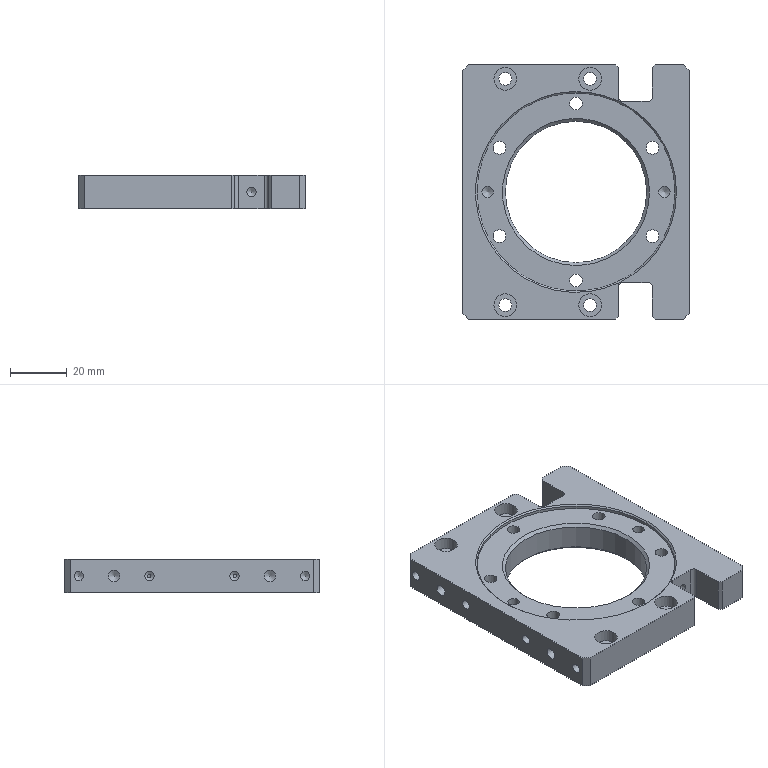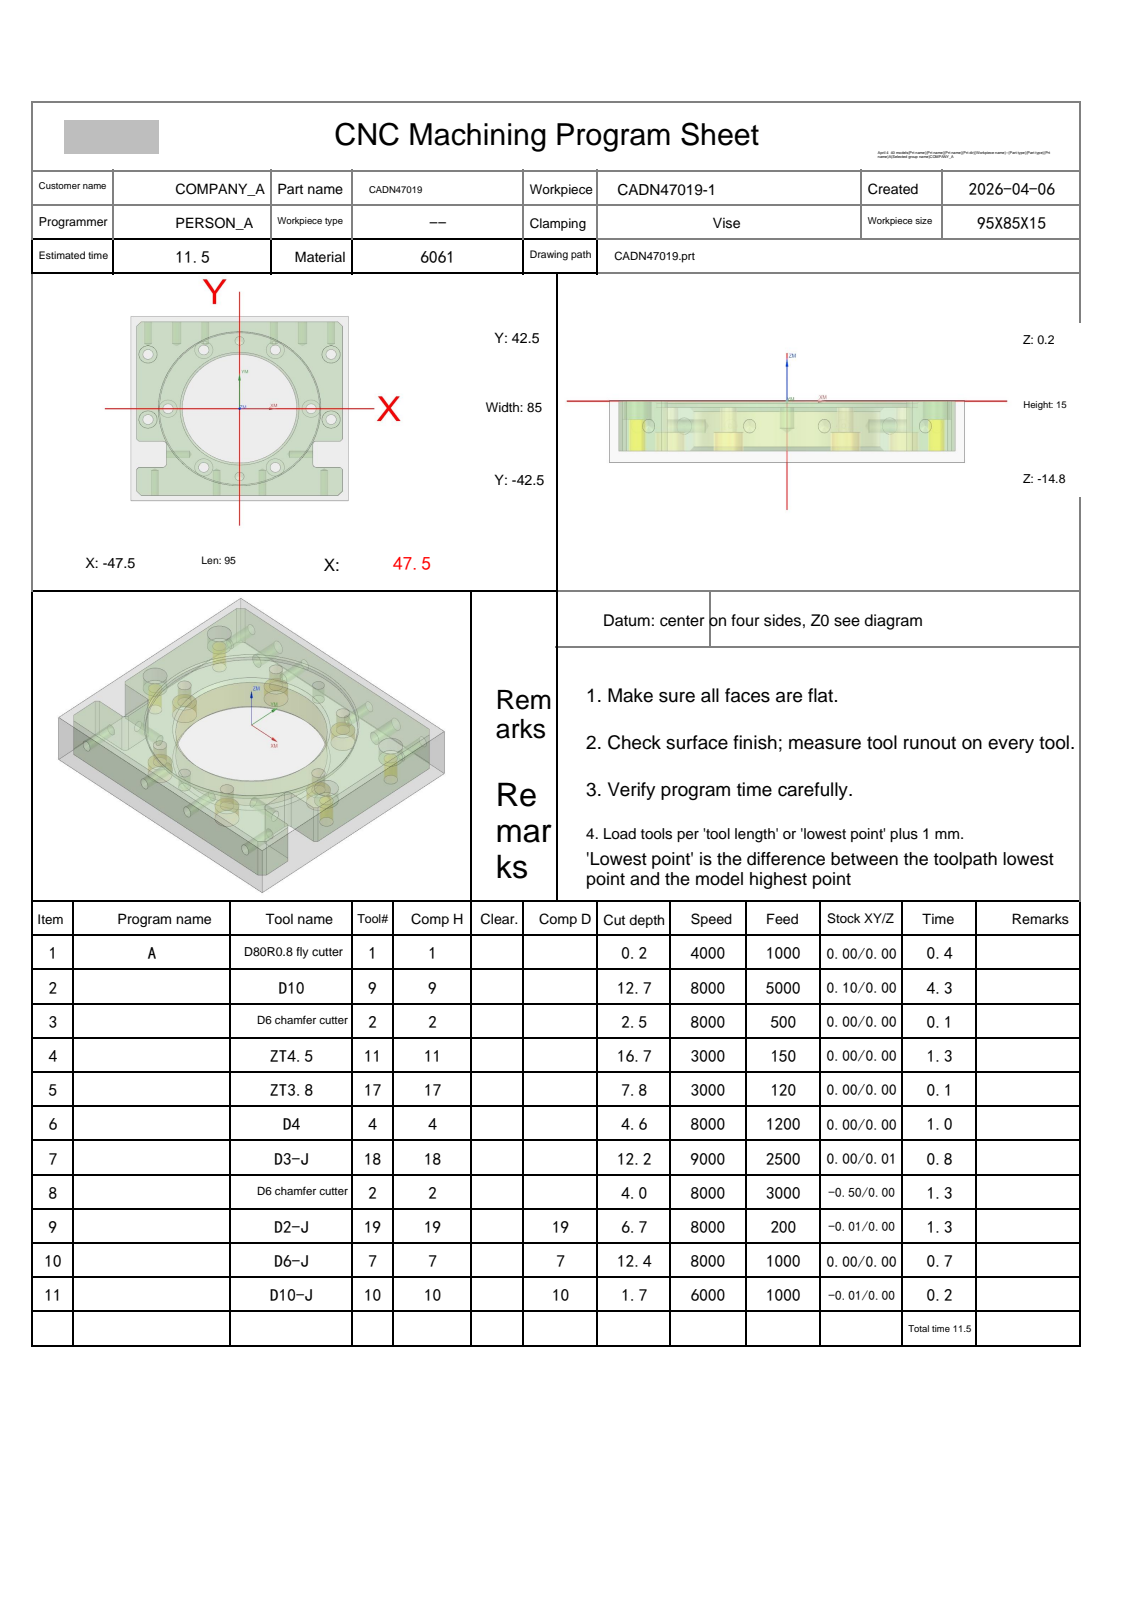NC program | NX | posted by the shop | part box 80 x 90 x 12 mm
Lines 6056 to 6628 of 6628:
N8 T02 M06
(D6 chamfer cutter  D=6. R=0. H=02 ce=0.00 di=0.00)
G00 G90 G54 X-.25 Y42.128 M03 S8000
G43 H02 Z20.
M08
Z2.099
G01 Z-1.5 F3000.
G03 X-.33 Y41.828 I.52 J-.3
X-.03 Y41.308 I.6 J0.0
G01 X0.0 Y41.3
X43.
X43.254 Y41.275
X43.497 Y41.201
X43.722 Y41.081
X43.919 Y40.919
X45.919 Y38.919
X46.081 Y38.722
X46.201 Y38.497
X46.275 Y38.254
X46.3 Y38.
Y-14.
X46.275 Y-14.254
X46.201 Y-14.497
X46.081 Y-14.722
X45.919 Y-14.919
X44.919 Y-15.919
X44.722 Y-16.081
X44.497 Y-16.201
X44.254 Y-16.275
X44. Y-16.3
X33.5
X33.4 Y-16.327
X33.327 Y-16.4
X33.3 Y-16.5
Y-25.5
X33.327 Y-25.6
X33.4 Y-25.673
X33.5 Y-25.7
X44.
X44.254 Y-25.725
X44.497 Y-25.799
X44.722 Y-25.919
X44.919 Y-26.081
X45.919 Y-27.081
X46.081 Y-27.278
X46.201 Y-27.503
X46.275 Y-27.746
X46.3 Y-28.
Y-38.
X46.275 Y-38.254
X46.201 Y-38.497
X46.081 Y-38.722
X45.919 Y-38.919
X43.919 Y-40.919
X43.722 Y-41.081
X43.497 Y-41.201
X43.254 Y-41.275
X43. Y-41.3
X-43.
X-43.254 Y-41.275
X-43.497 Y-41.201
X-43.722 Y-41.081
X-43.919 Y-40.919
X-45.919 Y-38.919
X-46.081 Y-38.722
X-46.201 Y-38.497
X-46.275 Y-38.254
X-46.3 Y-38.
Y-28.
X-46.275 Y-27.746
X-46.201 Y-27.503
X-46.081 Y-27.278
X-45.919 Y-27.081
X-44.919 Y-26.081
X-44.722 Y-25.919
X-44.497 Y-25.799
X-44.254 Y-25.725
X-44. Y-25.7
X-33.5
X-33.4 Y-25.673
X-33.327 Y-25.6
X-33.3 Y-25.5
Y-16.5
X-33.327 Y-16.4
X-33.4 Y-16.327
X-33.5 Y-16.3
X-44.
X-44.254 Y-16.275
X-44.497 Y-16.201
X-44.722 Y-16.081
X-44.919 Y-15.919
X-45.919 Y-14.919
X-46.081 Y-14.722
X-46.201 Y-14.497
X-46.275 Y-14.254
X-46.3 Y-14.
Y38.
X-46.275 Y38.254
X-46.201 Y38.497
X-46.081 Y38.722
X-45.919 Y38.919
X-43.919 Y40.919
X-43.722 Y41.081
X-43.497 Y41.201
X-43.254 Y41.275
X-43. Y41.3
X0.0
X.03 Y41.308
G03 X.33 Y41.828 I-.3 J.52
X.25 Y42.128 I-.6 J0.0
G01 Z2.099
G00 Z20.
G00 G90 X0.0 Y-31.25 M03 S8000
Z20.
G98 G81 X0.0 Y-31.25 Z-3.8 R1.5 F500.
Y31.25
G80
G00 Z20.
G00 G90 X-30.7 Y.018 M03 S8000
Z20.
Z-2.
G01 Z-2.5 F500.
X-29.75 Y.05
G03 X-31.25 Y1.55 I-1.5 J0.0
X-32.8 Y0.0 I0.0 J-1.55
X-31.25 Y-1.55 I1.55 J0.0
X-29.7 Y0.0 I0.0 J1.55
X-31.25 Y1.55 I-1.55 J0.0
X-32.75 Y.05 I0.0 J-1.5
G01 X-31.8 Y.018
Z-2.
G00 Z20.
X-15.075 Y-27.045
Z-2.
G01 Z-2.5
X-14.125 Y-27.013
G03 X-15.625 Y-25.513 I-1.5 J0.0
X-17.175 Y-27.063 I0.0 J-1.55
X-15.625 Y-28.613 I1.55 J0.0
X-14.075 Y-27.063 I0.0 J1.55
X-15.625 Y-25.513 I-1.55 J0.0
X-17.125 Y-27.013 I0.0 J-1.5
G01 X-16.175 Y-27.045
Z-2.
G00 Z20.
X16.175
Z-2.
G01 Z-2.5
X17.125 Y-27.013
G03 X15.625 Y-25.513 I-1.5 J0.0
X14.075 Y-27.063 I0.0 J-1.55
X15.625 Y-28.613 I1.55 J0.0
X17.175 Y-27.063 I0.0 J1.55
X15.625 Y-25.513 I-1.55 J0.0
X14.125 Y-27.013 I0.0 J-1.5
G01 X15.075 Y-27.045
Z-2.
G00 Z20.
X31.8 Y.018
Z-2.
G01 Z-2.5
X32.75 Y.05
G03 X31.25 Y1.55 I-1.5 J0.0
X29.7 Y0.0 I0.0 J-1.55
X31.25 Y-1.55 I1.55 J0.0
X32.8 Y0.0 I0.0 J1.55
X31.25 Y1.55 I-1.55 J0.0
X29.75 Y.05 I0.0 J-1.5
G01 X30.7 Y.018
Z-2.
G00 Z20.
X16.175 Y27.082
Z-2.
G01 Z-2.5
X17.125 Y27.113
G03 X15.625 Y28.613 I-1.5 J0.0
X14.075 Y27.063 I0.0 J-1.55
X15.625 Y25.513 I1.55 J0.0
X17.175 Y27.063 I0.0 J1.55
X15.625 Y28.613 I-1.55 J0.0
X14.125 Y27.113 I0.0 J-1.5
G01 X15.075 Y27.082
Z-2.
G00 Z20.
X-15.075
Z-2.
G01 Z-2.5
X-14.125 Y27.113
G03 X-15.625 Y28.613 I-1.5 J0.0
X-17.175 Y27.063 I0.0 J-1.55
X-15.625 Y25.513 I1.55 J0.0
X-14.075 Y27.063 I0.0 J1.55
X-15.625 Y28.613 I-1.55 J0.0
X-17.125 Y27.113 I0.0 J-1.5
G01 X-16.175 Y27.082
Z-2.
G00 Z20.
G00 G90 X39.253 Y28.212 M03 S8000
Z20.
Z2.5
G01 X39.038 Y28.16 Z2.42 F500.
X38.672 Y28.024 Z2.278
X38.325 Y27.847 Z2.136
X38.001 Y27.629 Z1.994
X37.705 Y27.375 Z1.852
X37.441 Y27.088 Z1.71
X37.212 Y26.772 Z1.568
X37.072 Y26.528 Z1.465
X36.912 Y26.172 Z1.323
X36.795 Y25.8 Z1.181
X36.723 Y25.416 Z1.039
X36.697 Y25.027 Z.897
X36.717 Y24.638 Z.755
X36.783 Y24.253 Z.613
X36.893 Y23.879 Z.471
X37.047 Y23.52 Z.329
X37.242 Y23.182 Z.187
X37.476 Y22.87 Z.045
X37.744 Y22.587 Z-.097
X38.045 Y22.338 Z-.239
X38.372 Y22.126 Z-.381
X38.722 Y21.954 Z-.523
X39.09 Y21.825 Z-.665
X39.471 Y21.74 Z-.807
X39.859 Y21.7 Z-.949
X40. Z-1.
G03 X43.3 Y25. I0.0 J3.3
X40. Y28.3 I-3.3 J0.0
X36.7 Y25. I0.0 J-3.3
X40. Y21.7 I3.3 J0.0
X40.498 Y21.738 I0.0 J3.3
G01 Z1.5
G00 Z20.
X39.253 Y-1.788
Z2.5
G01 X39.038 Y-1.84 Z2.42
X38.672 Y-1.976 Z2.278
X38.325 Y-2.153 Z2.136
X38.001 Y-2.371 Z1.994
X37.705 Y-2.625 Z1.852
X37.441 Y-2.912 Z1.71
X37.212 Y-3.228 Z1.568
X37.072 Y-3.472 Z1.465
X36.912 Y-3.828 Z1.323
X36.795 Y-4.2 Z1.181
X36.723 Y-4.584 Z1.039
X36.697 Y-4.973 Z.897
X36.717 Y-5.362 Z.755
X36.783 Y-5.747 Z.613
X36.893 Y-6.121 Z.471
X37.047 Y-6.48 Z.329
X37.242 Y-6.818 Z.187
X37.476 Y-7.13 Z.045
X37.744 Y-7.413 Z-.097
X38.045 Y-7.662 Z-.239
X38.372 Y-7.874 Z-.381
X38.722 Y-8.046 Z-.523
X39.09 Y-8.175 Z-.665
X39.471 Y-8.26 Z-.807
X39.859 Y-8.3 Z-.949
X40. Z-1.
G03 X43.3 Y-5. I0.0 J3.3
X40. Y-1.7 I-3.3 J0.0
X36.7 Y-5. I0.0 J-3.3
X40. Y-8.3 I3.3 J0.0
X40.498 Y-8.262 I0.0 J3.3
G01 Z1.5
G00 Z20.
X-40.747 Y-1.788
Z2.5
G01 X-40.962 Y-1.84 Z2.42
X-41.328 Y-1.976 Z2.278
X-41.675 Y-2.153 Z2.136
X-41.999 Y-2.371 Z1.994
X-42.295 Y-2.625 Z1.852
X-42.559 Y-2.912 Z1.71
X-42.788 Y-3.228 Z1.568
X-42.928 Y-3.472 Z1.465
X-43.088 Y-3.828 Z1.323
X-43.205 Y-4.2 Z1.181
X-43.277 Y-4.584 Z1.039
X-43.303 Y-4.973 Z.897
X-43.283 Y-5.362 Z.755
X-43.217 Y-5.747 Z.613
X-43.107 Y-6.121 Z.471
X-42.953 Y-6.48 Z.329
X-42.758 Y-6.818 Z.187
X-42.524 Y-7.13 Z.045
X-42.256 Y-7.413 Z-.097
X-41.955 Y-7.662 Z-.239
X-41.628 Y-7.874 Z-.381
X-41.278 Y-8.046 Z-.523
X-40.91 Y-8.175 Z-.665
X-40.529 Y-8.26 Z-.807
X-40.141 Y-8.3 Z-.949
X-40. Z-1.
G03 X-36.7 Y-5. I0.0 J3.3
X-40. Y-1.7 I-3.3 J0.0
X-43.3 Y-5. I0.0 J-3.3
X-40. Y-8.3 I3.3 J0.0
X-39.502 Y-8.262 I0.0 J3.3
G01 Z1.5
G00 Z20.
X-40.747 Y28.212
Z2.5
G01 X-40.962 Y28.16 Z2.42
X-41.328 Y28.024 Z2.278
X-41.675 Y27.847 Z2.136
X-41.999 Y27.629 Z1.994
X-42.295 Y27.375 Z1.852
X-42.559 Y27.088 Z1.71
X-42.788 Y26.772 Z1.568
X-42.928 Y26.528 Z1.465
X-43.088 Y26.172 Z1.323
X-43.205 Y25.8 Z1.181
X-43.277 Y25.416 Z1.039
X-43.303 Y25.027 Z.897
X-43.283 Y24.638 Z.755
X-43.217 Y24.253 Z.613
X-43.107 Y23.879 Z.471
X-42.953 Y23.52 Z.329
X-42.758 Y23.182 Z.187
X-42.524 Y22.87 Z.045
X-42.256 Y22.587 Z-.097
X-41.955 Y22.338 Z-.239
X-41.628 Y22.126 Z-.381
X-41.278 Y21.954 Z-.523
X-40.91 Y21.825 Z-.665
X-40.529 Y21.74 Z-.807
X-40.141 Y21.7 Z-.949
X-40. Z-1.
G03 X-36.7 Y25. I0.0 J3.3
X-40. Y28.3 I-3.3 J0.0
X-43.3 Y25. I0.0 J-3.3
X-40. Y21.7 I3.3 J0.0
X-39.502 Y21.738 I0.0 J3.3
G01 Z1.5
G00 Z20.
G00 G90 X3. Y31.5 M03 S8000
Z20.
Z-.5
G01 Z-1. F500.
G03 X0.0 Y34.5 I-3. J0.0
X-34.5 Y0.0 I0.0 J-34.5
X0.0 Y-34.5 I34.5 J0.0
X34.5 Y0.0 I0.0 J34.5
X0.0 Y34.5 I-34.5 J0.0
X-3. Y31.5 I0.0 J-3.
G01 Z-.5
G00 Z20.
G00 G90 X1.2 Y23.069 M03 S6500
Z20.
Z-1.7
G01 Z-3.2 F1500.
Y23.1
G03 X0.0 Y24.3 I-1.2 J0.0
X-24.3 Y0.0 I0.0 J-24.3
X0.0 Y-24.3 I24.3 J0.0
X23.42 Y-6.479 I0.0 J24.3
X23.65 Y-5.583 I-23.42 J6.479
X23.928 Y-4.235 I-23.65 J5.583
X24.051 Y-3.471 I-23.928 J4.235
X24.21 Y-2.09 I-24.051 J3.471
X24.228 Y-1.866 I-24.21 J2.09
X24.3 Y0.0 I-24.228 J1.866
X0.0 Y24.3 I-24.3 J0.0
X-.4 Y24.297 I0.0 J-24.3
X-1.58 Y23.097 I.02 J-1.2
G01 Y23.077
Y23.046
Z-1.7
G00 Z20.
G91 G28 Z0.0
M05
M09
G91 G28 Z0.0
M01
N9 T19 M06
(D2-J  D=2. R=0. H=19 ce=-0.01 di=0.00)
G00 G90 G54 X0.0 Y-31.25 M03 S8000
G43 H19 Z20.
M08
Z-1.
G41 D19
G01 X-.185 Y-31.326 F200.
G03 X-.485 Y-31.775 I.185 J-.449
X0.0 Y-32.26 I.485 J0.0
X0.0 Y-32.26 Z-1.3 I0.0 J1.01
X0.0 Y-32.26 Z-1.6 I0.0 J1.01
X0.0 Y-32.26 Z-1.9 I0.0 J1.01
X0.0 Y-32.26 Z-2.2 I0.0 J1.01
X0.0 Y-32.26 Z-2.5 I0.0 J1.01
X0.0 Y-32.26 Z-2.8 I0.0 J1.01
X0.0 Y-32.26 Z-3.1 I0.0 J1.01
X0.0 Y-32.26 Z-3.4 I0.0 J1.01
X0.0 Y-32.26 Z-3.7 I0.0 J1.01
X0.0 Y-32.26 Z-4. I0.0 J1.01
X0.0 Y-32.26 Z-4.3 I0.0 J1.01
X0.0 Y-32.26 Z-4.6 I0.0 J1.01
X0.0 Y-32.26 Z-4.9 I0.0 J1.01
X0.0 Y-32.26 Z-5.2 I0.0 J1.01
X0.0 Y-32.26 Z-5.5 I0.0 J1.01
X0.0 Y-32.26 Z-5.8 I0.0 J1.01
X0.0 Y-32.26 Z-6.1 I0.0 J1.01
X0.0 Y-32.26 Z-6.4 I0.0 J1.01
X.875 Y-30.745 Z-6.5 I0.0 J1.01
X0.0 Y-30.24 I-.875 J-.505
X-1.01 Y-31.25 I0.0 J-1.01
X0.0 Y-32.26 I1.01 J0.0
X1.01 Y-31.25 I0.0 J1.01
X.875 Y-30.745 I-1.01 J0.0
X.454 Y-30.502 I-.42 J-.243
X-.031 Y-30.988 I0.0 J-.485
G01 X-.026 Y-31.052
G40 X0.0 Y-31.25
G00 Z20.
Y31.25
Z-1.
G41 D19
G01 X-.185 Y31.174
G03 X-.485 Y30.725 I.185 J-.449
X0.0 Y30.24 I.485 J0.0
X0.0 Y30.24 Z-1.3 I0.0 J1.01
X0.0 Y30.24 Z-1.6 I0.0 J1.01
X0.0 Y30.24 Z-1.9 I0.0 J1.01
X0.0 Y30.24 Z-2.2 I0.0 J1.01
X0.0 Y30.24 Z-2.5 I0.0 J1.01
X0.0 Y30.24 Z-2.8 I0.0 J1.01
X0.0 Y30.24 Z-3.1 I0.0 J1.01
X0.0 Y30.24 Z-3.4 I0.0 J1.01
X0.0 Y30.24 Z-3.7 I0.0 J1.01
X0.0 Y30.24 Z-4. I0.0 J1.01
X0.0 Y30.24 Z-4.3 I0.0 J1.01
X0.0 Y30.24 Z-4.6 I0.0 J1.01
X0.0 Y30.24 Z-4.9 I0.0 J1.01
X0.0 Y30.24 Z-5.2 I0.0 J1.01
X0.0 Y30.24 Z-5.5 I0.0 J1.01
X0.0 Y30.24 Z-5.8 I0.0 J1.01
X0.0 Y30.24 Z-6.1 I0.0 J1.01
X0.0 Y30.24 Z-6.4 I0.0 J1.01
X.875 Y31.755 Z-6.5 I0.0 J1.01
X0.0 Y32.26 I-.875 J-.505
X-1.01 Y31.25 I0.0 J-1.01
X0.0 Y30.24 I1.01 J0.0
X1.01 Y31.25 I0.0 J1.01
X.875 Y31.755 I-1.01 J0.0
X.454 Y31.998 I-.42 J-.243
X-.031 Y31.512 I0.0 J-.485
G01 X-.026 Y31.448
G40 X0.0 Y31.25
G00 Z20.
G91 G28 Z0.0
M05
M09
G91 G28 Z0.0
M01
N10 T07 M06
(D6-J  D=6. R=0. H=07 ce=0.00 di=0.00)
G00 G90 G54 X.9 Y20.881 M03 S8000
G43 H07 Z10.2
M08
Z-5.75
G01 Z-7.25 F1000.
G41 D07
Y21.1
G03 X0.0 Y22. I-.9 J0.0
X-22. Y0.0 I0.0 J-22.
X0.0 Y-22. I22. J0.0
X22. Y0.0 I0.0 J22.
X0.0 Y22. I-22. J0.0
X-.4 Y21.996 I0.0 J-22.
X-1.284 Y21.097 I.016 J-.9
G01 X-1.283 Y21.08
Y21.061
G40 X-1.279 Y20.861
Z-5.75
G00 X.9 Y20.881
Z-10.5
G01 Z-12.
G41 D07
Y21.1
G03 X0.0 Y22. I-.9 J0.0
X-22. Y0.0 I0.0 J-22.
X0.0 Y-22. I22. J0.0
X22. Y0.0 I0.0 J22.
X0.0 Y22. I-22. J0.0
X-.4 Y21.996 I0.0 J-22.
X-1.284 Y21.097 I.016 J-.9
G01 X-1.283 Y21.08
Y21.061
G40 X-1.279 Y20.861
Z-10.5
G00 Z10.2
G00 G90 X44.017 Y-44.073 M03 S8000
Z20.
Z-11.7
G01 Z-12.2 F1000.
G41 D07
X43.992 Y-43.875
G03 X43. Y-43. I-.992 J-.125
G01 X-43.
G02 X-45.121 Y-42.121 I0.0 J3.
G01 X-47.121 Y-40.121
G02 X-48. Y-38. I2.121 J2.121
G01 Y-28.
G02 X-47.121 Y-25.879 I3. J0.0
G01 X-46.121 Y-24.879
G02 X-44. Y-24. I2.121 J-2.121
G01 X-35.
Y-18.
X-44.
G02 X-46.121 Y-17.121 I0.0 J3.
G01 X-47.121 Y-16.121
G02 X-48. Y-14. I2.121 J2.121
G01 Y38.
G02 X-47.121 Y40.121 I3. J0.0
G01 X-45.121 Y42.121
G02 X-43. Y43. I2.121 J-2.121
G01 X43.
G02 X45.121 Y42.121 I0.0 J-3.
G01 X47.121 Y40.121
G02 X48. Y38. I-2.121 J-2.121
G01 Y-14.
G02 X47.121 Y-16.121 I-3. J0.0
G01 X46.121 Y-17.121
G02 X44. Y-18. I-2.121 J2.121
G01 X35.
Y-24.
X44.
G02 X46.121 Y-24.879 I0.0 J-3.
G01 X47.121 Y-25.879
G02 X48. Y-28. I-2.121 J-2.121
G01 Y-38.
G02 X47.121 Y-40.121 I-3. J0.0
G01 X45.121 Y-42.121
G02 X43. Y-43. I-2.121 J2.121
G01 X42.5
G03 X41.5 Y-44. I0.0 J-1.
G01 G40 Y-44.2
Z-11.7
G00 Z20.
G91 G28 Z0.0
M05
M09
G91 G28 Z0.0
M01
N11 T10 M06
(D10-J  D=10. R=0. H=10 ce=-0.01 di=0.00)
G00 G90 G54 X2. Y19.71 M03 S6000
G43 H10 Z10.2
M08
Z-.5
G01 Z-1.5 F1000.
G41 D10
Y28.01
G03 X0.0 Y30.01 I-2. J0.0
X-30.01 Y0.0 I0.0 J-30.01
X0.0 Y-30.01 I30.01 J0.0
X30.01 Y0.0 I0.0 J30.01
X0.0 Y30.01 I-30.01 J0.0
X-.4 Y30.007 I0.0 J-30.01
X-2.373 Y28.008 I.027 J-2.
G01 Y27.981
X-2.265 Y19.881
G40 X-2.263 Y19.681
Z-.5
G00 Z10.2
M05
M09
G91 G28 Z0.0
G91 G28 Y0.0
M30
%